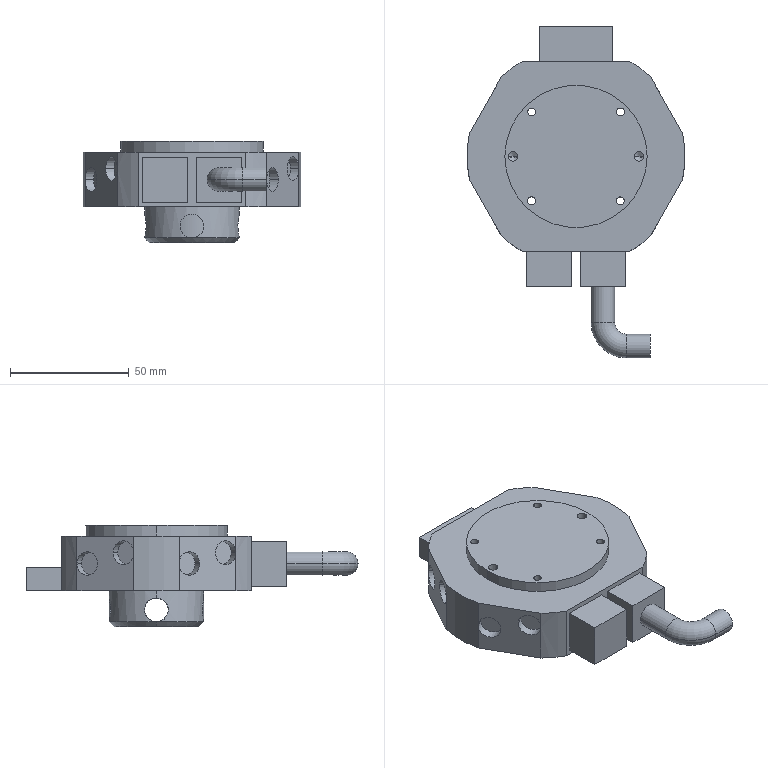Part | SolidWorks | features ICE 1, MBimport 1 | 1 solid | 96 faces | box 92 x 140 x 42.6 mm | volume 179973 mm3 | cylinder 54 | plane 34 | cone 6 | torus 2 | commonest cylinder face diameters 10 x28 3.3 x8 92 x6 4 x4 40 x4 20 x2